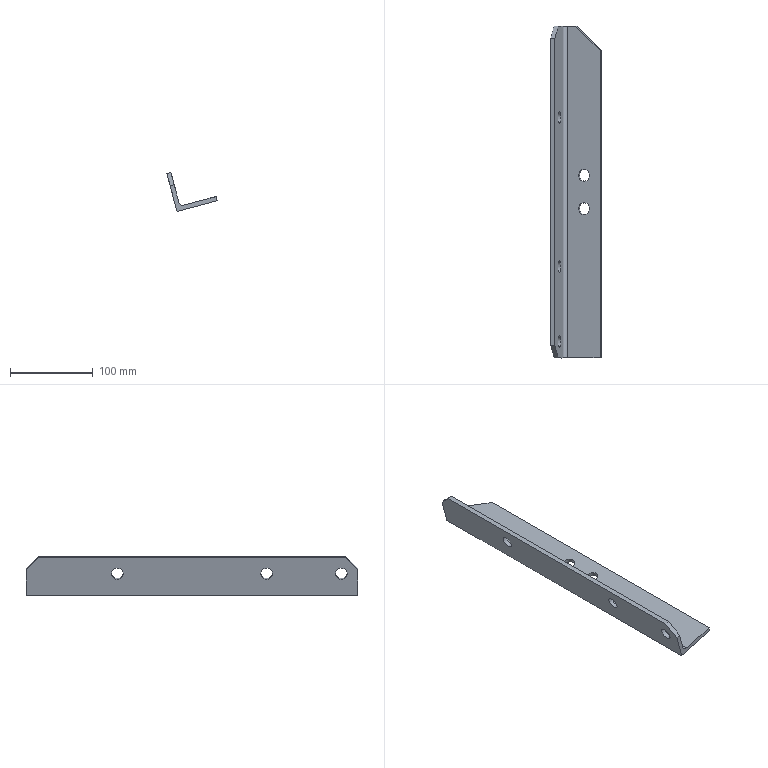Part | NX | features solid 2 | 1 solid | 17 faces | box 60.461 x 400 x 46.693 mm | volume 178923 mm3 | plane 11 | cylinder 6 | commonest cylinder face diameters 14 x5 10 x1
STEP:
#1=CARTESIAN_POINT('',(712.611,-855.,-13.897));
#2=VERTEX_POINT('',#1);
#3=CARTESIAN_POINT('',(719.373,-855.,-12.085));
#4=DIRECTION('',(0.2588,0.,-0.9659));
#5=DIRECTION('',(-0.9659,0.,-0.2588));
#6=AXIS2_PLACEMENT_3D('',#3,#4,#5);
#7=CIRCLE('',#6,7.);
#8=EDGE_CURVE('',#2,#2,#7,.T.);
#9=ORIENTED_EDGE('',*,*,#8,.T.);
#10=EDGE_LOOP('',(#9));
#11=FACE_BOUND('',#10,.T.);
#12=CARTESIAN_POINT('',(738.691,-665.,-6.909));
#13=VERTEX_POINT('',#12);
#14=CARTESIAN_POINT('',(738.691,-1035.,-6.909));
#15=VERTEX_POINT('',#14);
#16=CARTESIAN_POINT('',(738.691,-859.636,-6.909));
#17=DIRECTION('',(0.,-1.,0.));
#18=VECTOR('',#17,1000.);
#19=LINE('',#16,#18);
#20=EDGE_CURVE('',#13,#15,#19,.T.);
#21=ORIENTED_EDGE('',*,*,#20,.F.);
#22=CARTESIAN_POINT('',(709.713,-635.,-14.673));
#23=VERTEX_POINT('',#22);
#24=CARTESIAN_POINT('',(831.809,-761.403,18.042));
#25=DIRECTION('',(0.683,-0.7071,0.183));
#26=VECTOR('',#25,1000.);
#27=LINE('',#24,#26);
#28=EDGE_CURVE('',#13,#23,#27,.F.);
#29=ORIENTED_EDGE('',*,*,#28,.T.);
#30=CARTESIAN_POINT('',(700.054,-635.,-17.261));
#31=VERTEX_POINT('',#30);
#32=CARTESIAN_POINT('',(695.225,-635.,-18.555));
#33=DIRECTION('',(-0.9659,0.,-0.2588));
#34=VECTOR('',#33,1000.);
#35=LINE('',#32,#34);
#36=EDGE_CURVE('',#23,#31,#35,.T.);
#37=ORIENTED_EDGE('',*,*,#36,.T.);
#38=CARTESIAN_POINT('',(700.054,-1035.,-17.261));
#39=VERTEX_POINT('',#38);
#40=CARTESIAN_POINT('',(700.054,-740.,-17.261));
#41=DIRECTION('',(0.,-1.,0.));
#42=VECTOR('',#41,1000.);
#43=LINE('',#40,#42);
#44=EDGE_CURVE('',#39,#31,#43,.F.);
#45=ORIENTED_EDGE('',*,*,#44,.F.);
#46=CARTESIAN_POINT('',(738.691,-1035.,-6.909));
#47=DIRECTION('',(0.9659,0.,0.2588));
#48=VECTOR('',#47,1000.);
#49=LINE('',#46,#48);
#50=EDGE_CURVE('',#39,#15,#49,.T.);
#51=ORIENTED_EDGE('',*,*,#50,.T.);
#52=EDGE_LOOP('',(#21,#29,#37,#45,#51));
#53=FACE_BOUND('',#52,.T.);
#54=CARTESIAN_POINT('',(712.611,-815.,-13.897));
#55=VERTEX_POINT('',#54);
#56=CARTESIAN_POINT('',(719.373,-815.,-12.085));
#57=DIRECTION('',(0.2588,0.,-0.9659));
#58=DIRECTION('',(-0.9659,0.,-0.2588));
#59=AXIS2_PLACEMENT_3D('',#56,#57,#58);
#60=CIRCLE('',#59,7.);
#61=EDGE_CURVE('',#55,#55,#60,.T.);
#62=ORIENTED_EDGE('',*,*,#61,.T.);
#63=EDGE_LOOP('',(#62));
#64=FACE_BOUND('',#63,.T.);
#65=CARTESIAN_POINT('',(738.691,-857.805,-6.909));
#66=DIRECTION('',(-0.2588,0.,0.9659));
#67=DIRECTION('',(0.,-1.,0.));
#68=AXIS2_PLACEMENT_3D('',#65,#66,#67);
#69=PLANE('',#68);
#70=ADVANCED_FACE('',(#11,#53,#64),#69,.T.);
#71=CARTESIAN_POINT('',(713.905,-855.,-18.726));
#72=VERTEX_POINT('',#71);
#73=CARTESIAN_POINT('',(720.667,-855.,-16.915));
#74=DIRECTION('',(0.2588,0.,-0.9659));
#75=DIRECTION('',(-0.9659,0.,-0.2588));
#76=AXIS2_PLACEMENT_3D('',#73,#74,#75);
#77=CIRCLE('',#76,7.);
#78=EDGE_CURVE('',#72,#72,#77,.F.);
#79=ORIENTED_EDGE('',*,*,#78,.T.);
#80=EDGE_LOOP('',(#79));
#81=FACE_BOUND('',#80,.T.);
#82=CARTESIAN_POINT('',(691.689,-635.,-24.679));
#83=VERTEX_POINT('',#82);
#84=CARTESIAN_POINT('',(711.008,-635.,-19.503));
#85=VERTEX_POINT('',#84);
#86=CARTESIAN_POINT('',(696.519,-635.,-23.385));
#87=DIRECTION('',(0.9659,0.,0.2588));
#88=VECTOR('',#87,1000.);
#89=LINE('',#86,#88);
#90=EDGE_CURVE('',#83,#85,#89,.T.);
#91=ORIENTED_EDGE('',*,*,#90,.T.);
#92=CARTESIAN_POINT('',(739.985,-665.,-11.738));
#93=VERTEX_POINT('',#92);
#94=CARTESIAN_POINT('',(811.222,-738.75,7.35));
#95=DIRECTION('',(-0.683,0.7071,-0.183));
#96=VECTOR('',#95,1000.);
#97=LINE('',#94,#96);
#98=EDGE_CURVE('',#85,#93,#97,.F.);
#99=ORIENTED_EDGE('',*,*,#98,.T.);
#100=CARTESIAN_POINT('',(739.985,-1035.,-11.738));
#101=VERTEX_POINT('',#100);
#102=CARTESIAN_POINT('',(739.985,-857.5,-11.738));
#103=DIRECTION('',(0.,-1.,0.));
#104=VECTOR('',#103,1000.);
#105=LINE('',#102,#104);
#106=EDGE_CURVE('',#93,#101,#105,.T.);
#107=ORIENTED_EDGE('',*,*,#106,.T.);
#108=CARTESIAN_POINT('',(691.689,-1035.,-24.679));
#109=VERTEX_POINT('',#108);
#110=CARTESIAN_POINT('',(696.519,-1035.,-23.385));
#111=DIRECTION('',(-0.9659,0.,-0.2588));
#112=VECTOR('',#111,1000.);
#113=LINE('',#110,#112);
#114=EDGE_CURVE('',#101,#109,#113,.T.);
#115=ORIENTED_EDGE('',*,*,#114,.T.);
#116=CARTESIAN_POINT('',(691.689,-859.636,-24.679));
#117=DIRECTION('',(0.,-1.,0.));
#118=VECTOR('',#117,1000.);
#119=LINE('',#116,#118);
#120=EDGE_CURVE('',#83,#109,#119,.T.);
#121=ORIENTED_EDGE('',*,*,#120,.F.);
#122=EDGE_LOOP('',(#91,#99,#107,#115,#121));
#123=FACE_BOUND('',#122,.T.);
#124=CARTESIAN_POINT('',(713.905,-815.,-18.726));
#125=VERTEX_POINT('',#124);
#126=CARTESIAN_POINT('',(720.667,-815.,-16.915));
#127=DIRECTION('',(0.2588,0.,-0.9659));
#128=DIRECTION('',(-0.9659,0.,-0.2588));
#129=AXIS2_PLACEMENT_3D('',#126,#127,#128);
#130=CIRCLE('',#129,7.);
#131=EDGE_CURVE('',#125,#125,#130,.F.);
#132=ORIENTED_EDGE('',*,*,#131,.T.);
#133=EDGE_LOOP('',(#132));
#134=FACE_BOUND('',#133,.T.);
#135=CARTESIAN_POINT('',(696.519,-857.5,-23.385));
#136=DIRECTION('',(0.2588,0.,-0.9659));
#137=DIRECTION('',(0.,1.,0.));
#138=AXIS2_PLACEMENT_3D('',#135,#136,#137);
#139=PLANE('',#138);
#140=ADVANCED_FACE('',(#81,#123,#134),#139,.T.);
#141=CARTESIAN_POINT('',(691.342,-745.,-4.067));
#142=VERTEX_POINT('',#141);
#143=CARTESIAN_POINT('',(689.531,-745.,2.695));
#144=DIRECTION('',(0.9659,0.,0.2588));
#145=DIRECTION('',(0.2588,0.,-0.9659));
#146=AXIS2_PLACEMENT_3D('',#143,#144,#145);
#147=CIRCLE('',#146,7.);
#148=EDGE_CURVE('',#142,#142,#147,.F.);
#149=ORIENTED_EDGE('',*,*,#148,.T.);
#150=EDGE_LOOP('',(#149));
#151=FACE_BOUND('',#150,.T.);
#152=CARTESIAN_POINT('',(691.342,-925.,-4.067));
#153=VERTEX_POINT('',#152);
#154=CARTESIAN_POINT('',(689.531,-925.,2.695));
#155=DIRECTION('',(0.9659,0.,0.2588));
#156=DIRECTION('',(0.2588,0.,-0.9659));
#157=AXIS2_PLACEMENT_3D('',#154,#155,#156);
#158=CIRCLE('',#157,7.);
#159=EDGE_CURVE('',#153,#153,#158,.F.);
#160=ORIENTED_EDGE('',*,*,#159,.T.);
#161=EDGE_LOOP('',(#160));
#162=FACE_BOUND('',#161,.T.);
#163=CARTESIAN_POINT('',(688.236,-1035.,7.525));
#164=VERTEX_POINT('',#163);
#165=CARTESIAN_POINT('',(693.93,-1035.,-13.726));
#166=VERTEX_POINT('',#165);
#167=CARTESIAN_POINT('',(687.46,-1035.,10.422));
#168=DIRECTION('',(0.2588,0.,-0.9659));
#169=VECTOR('',#168,1000.);
#170=LINE('',#167,#169);
#171=EDGE_CURVE('',#164,#166,#170,.T.);
#172=ORIENTED_EDGE('',*,*,#171,.T.);
#173=CARTESIAN_POINT('',(693.93,-635.,-13.726));
#174=VERTEX_POINT('',#173);
#175=CARTESIAN_POINT('',(693.93,-1074.813,-13.726));
#176=DIRECTION('',(0.,-1.,0.));
#177=VECTOR('',#176,1000.);
#178=LINE('',#175,#177);
#179=EDGE_CURVE('',#174,#166,#178,.T.);
#180=ORIENTED_EDGE('',*,*,#179,.F.);
#181=CARTESIAN_POINT('',(688.236,-635.,7.525));
#182=VERTEX_POINT('',#181);
#183=CARTESIAN_POINT('',(689.531,-635.,2.695));
#184=DIRECTION('',(-0.2588,0.,0.9659));
#185=VECTOR('',#184,1000.);
#186=LINE('',#183,#185);
#187=EDGE_CURVE('',#174,#182,#186,.T.);
#188=ORIENTED_EDGE('',*,*,#187,.T.);
#189=CARTESIAN_POINT('',(684.354,-650.,22.013));
#190=VERTEX_POINT('',#189);
#191=CARTESIAN_POINT('',(670.425,-703.818,73.997));
#192=DIRECTION('',(-0.183,-0.7071,0.683));
#193=VECTOR('',#192,1000.);
#194=LINE('',#191,#193);
#195=EDGE_CURVE('',#190,#182,#194,.F.);
#196=ORIENTED_EDGE('',*,*,#195,.F.);
#197=CARTESIAN_POINT('',(684.354,-1020.,22.013));
#198=VERTEX_POINT('',#197);
#199=CARTESIAN_POINT('',(684.354,-859.636,22.013));
#200=DIRECTION('',(0.,-1.,0.));
#201=VECTOR('',#200,1000.);
#202=LINE('',#199,#201);
#203=EDGE_CURVE('',#190,#198,#202,.T.);
#204=ORIENTED_EDGE('',*,*,#203,.T.);
#205=CARTESIAN_POINT('',(665.154,-945.818,93.668));
#206=DIRECTION('',(-0.183,0.7071,0.683));
#207=VECTOR('',#206,1000.);
#208=LINE('',#205,#207);
#209=EDGE_CURVE('',#164,#198,#208,.T.);
#210=ORIENTED_EDGE('',*,*,#209,.F.);
#211=EDGE_LOOP('',(#172,#180,#188,#196,#204,#210));
#212=FACE_BOUND('',#211,.T.);
#213=CARTESIAN_POINT('',(687.719,-1015.,9.456));
#214=VERTEX_POINT('',#213);
#215=CARTESIAN_POINT('',(689.531,-1015.,2.695));
#216=DIRECTION('',(-0.9659,0.,-0.2588));
#217=DIRECTION('',(-0.2588,0.,0.9659));
#218=AXIS2_PLACEMENT_3D('',#215,#216,#217);
#219=CIRCLE('',#218,7.);
#220=EDGE_CURVE('',#214,#214,#219,.F.);
#221=ORIENTED_EDGE('',*,*,#220,.F.);
#222=EDGE_LOOP('',(#221));
#223=FACE_BOUND('',#222,.T.);
#224=CARTESIAN_POINT('',(687.46,-859.636,10.422));
#225=DIRECTION('',(0.9659,0.,0.2588));
#226=DIRECTION('',(0.2588,0.,-0.9659));
#227=AXIS2_PLACEMENT_3D('',#224,#225,#226);
#228=PLANE('',#227);
#229=ADVANCED_FACE('',(#151,#162,#212,#223),#228,.T.);
#230=CARTESIAN_POINT('',(682.889,-745.,8.162));
#231=VERTEX_POINT('',#230);
#232=CARTESIAN_POINT('',(684.701,-745.,1.401));
#233=DIRECTION('',(-0.9659,0.,-0.2588));
#234=DIRECTION('',(-0.2588,0.,0.9659));
#235=AXIS2_PLACEMENT_3D('',#232,#233,#234);
#236=CIRCLE('',#235,7.);
#237=EDGE_CURVE('',#231,#231,#236,.F.);
#238=ORIENTED_EDGE('',*,*,#237,.T.);
#239=EDGE_LOOP('',(#238));
#240=FACE_BOUND('',#239,.T.);
#241=CARTESIAN_POINT('',(682.889,-925.,8.162));
#242=VERTEX_POINT('',#241);
#243=CARTESIAN_POINT('',(684.701,-925.,1.401));
#244=DIRECTION('',(-0.9659,0.,-0.2588));
#245=DIRECTION('',(-0.2588,0.,0.9659));
#246=AXIS2_PLACEMENT_3D('',#243,#244,#245);
#247=CIRCLE('',#246,7.);
#248=EDGE_CURVE('',#242,#242,#247,.F.);
#249=ORIENTED_EDGE('',*,*,#248,.T.);
#250=EDGE_LOOP('',(#249));
#251=FACE_BOUND('',#250,.T.);
#252=CARTESIAN_POINT('',(679.525,-650.,20.719));
#253=VERTEX_POINT('',#252);
#254=CARTESIAN_POINT('',(679.525,-1020.,20.719));
#255=VERTEX_POINT('',#254);
#256=CARTESIAN_POINT('',(679.525,-859.636,20.719));
#257=DIRECTION('',(0.,-1.,0.));
#258=VECTOR('',#257,1000.);
#259=LINE('',#256,#258);
#260=EDGE_CURVE('',#253,#255,#259,.T.);
#261=ORIENTED_EDGE('',*,*,#260,.F.);
#262=CARTESIAN_POINT('',(683.407,-635.,6.23));
#263=VERTEX_POINT('',#262);
#264=CARTESIAN_POINT('',(665.595,-703.818,72.703));
#265=DIRECTION('',(0.183,0.7071,-0.683));
#266=VECTOR('',#265,1000.);
#267=LINE('',#264,#266);
#268=EDGE_CURVE('',#263,#253,#267,.F.);
#269=ORIENTED_EDGE('',*,*,#268,.F.);
#270=CARTESIAN_POINT('',(684.701,-635.,1.401));
#271=DIRECTION('',(0.2588,0.,-0.9659));
#272=VECTOR('',#271,1000.);
#273=LINE('',#270,#272);
#274=EDGE_CURVE('',#263,#83,#273,.T.);
#275=ORIENTED_EDGE('',*,*,#274,.T.);
#276=ORIENTED_EDGE('',*,*,#120,.T.);
#277=CARTESIAN_POINT('',(683.407,-1035.,6.23));
#278=VERTEX_POINT('',#277);
#279=CARTESIAN_POINT('',(682.63,-1035.,9.128));
#280=DIRECTION('',(-0.2588,0.,0.9659));
#281=VECTOR('',#280,1000.);
#282=LINE('',#279,#281);
#283=EDGE_CURVE('',#109,#278,#282,.T.);
#284=ORIENTED_EDGE('',*,*,#283,.T.);
#285=CARTESIAN_POINT('',(660.325,-945.818,92.374));
#286=DIRECTION('',(0.183,-0.7071,-0.683));
#287=VECTOR('',#286,1000.);
#288=LINE('',#285,#287);
#289=EDGE_CURVE('',#255,#278,#288,.T.);
#290=ORIENTED_EDGE('',*,*,#289,.F.);
#291=EDGE_LOOP('',(#261,#269,#275,#276,#284,#290));
#292=FACE_BOUND('',#291,.T.);
#293=CARTESIAN_POINT('',(686.513,-1015.,-5.361));
#294=VERTEX_POINT('',#293);
#295=CARTESIAN_POINT('',(684.701,-1015.,1.401));
#296=DIRECTION('',(0.9659,0.,0.2588));
#297=DIRECTION('',(0.2588,0.,-0.9659));
#298=AXIS2_PLACEMENT_3D('',#295,#296,#297);
#299=CIRCLE('',#298,7.);
#300=EDGE_CURVE('',#294,#294,#299,.T.);
#301=ORIENTED_EDGE('',*,*,#300,.T.);
#302=EDGE_LOOP('',(#301));
#303=FACE_BOUND('',#302,.T.);
#304=CARTESIAN_POINT('',(682.63,-859.636,9.128));
#305=DIRECTION('',(-0.9659,0.,-0.2588));
#306=DIRECTION('',(-0.2588,0.,0.9659));
#307=AXIS2_PLACEMENT_3D('',#304,#305,#306);
#308=PLANE('',#307);
#309=ADVANCED_FACE('',(#240,#251,#292,#303),#308,.T.);
#310=ORIENTED_EDGE('',*,*,#203,.F.);
#311=CARTESIAN_POINT('',(689.184,-650.,23.308));
#312=DIRECTION('',(0.9659,0.,0.2588));
#313=VECTOR('',#312,1000.);
#314=LINE('',#311,#313);
#315=EDGE_CURVE('',#253,#190,#314,.T.);
#316=ORIENTED_EDGE('',*,*,#315,.F.);
#317=ORIENTED_EDGE('',*,*,#260,.T.);
#318=CARTESIAN_POINT('',(679.525,-1020.,20.719));
#319=DIRECTION('',(-0.9659,0.,-0.2588));
#320=VECTOR('',#319,1000.);
#321=LINE('',#318,#320);
#322=EDGE_CURVE('',#198,#255,#321,.T.);
#323=ORIENTED_EDGE('',*,*,#322,.F.);
#324=EDGE_LOOP('',(#310,#316,#317,#323));
#325=FACE_BOUND('',#324,.T.);
#326=CARTESIAN_POINT('',(689.184,-859.636,23.308));
#327=DIRECTION('',(-0.2588,0.,0.9659));
#328=DIRECTION('',(0.,-1.,0.));
#329=AXIS2_PLACEMENT_3D('',#326,#327,#328);
#330=PLANE('',#329);
#331=ADVANCED_FACE('',(#325),#330,.T.);
#332=ORIENTED_EDGE('',*,*,#44,.T.);
#333=CARTESIAN_POINT('',(698.76,-635.,-12.432));
#334=DIRECTION('',(0.,-1.,0.));
#335=DIRECTION('',(0.9848,0.,-0.1736));
#336=AXIS2_PLACEMENT_3D('',#333,#334,#335);
#337=CIRCLE('',#336,5.);
#338=EDGE_CURVE('',#174,#31,#337,.T.);
#339=ORIENTED_EDGE('',*,*,#338,.F.);
#340=ORIENTED_EDGE('',*,*,#179,.T.);
#341=CARTESIAN_POINT('',(698.76,-1035.,-12.432));
#342=DIRECTION('',(0.,-1.,0.));
#343=DIRECTION('',(0.1736,0.,0.9848));
#344=AXIS2_PLACEMENT_3D('',#341,#342,#343);
#345=CIRCLE('',#344,5.);
#346=EDGE_CURVE('',#39,#166,#345,.F.);
#347=ORIENTED_EDGE('',*,*,#346,.F.);
#348=EDGE_LOOP('',(#332,#339,#340,#347));
#349=FACE_BOUND('',#348,.T.);
#350=CARTESIAN_POINT('',(698.76,-859.636,-12.432));
#351=DIRECTION('',(0.,1.,0.));
#352=DIRECTION('',(0.2588,0.,-0.9659));
#353=AXIS2_PLACEMENT_3D('',#350,#351,#352);
#354=CYLINDRICAL_SURFACE('',#353,5.);
#355=ADVANCED_FACE('',(#349),#354,.F.);
#356=ORIENTED_EDGE('',*,*,#106,.F.);
#357=CARTESIAN_POINT('',(730.927,-665.,22.069));
#358=DIRECTION('',(-0.2588,0.,0.9659));
#359=VECTOR('',#358,1000.);
#360=LINE('',#357,#359);
#361=EDGE_CURVE('',#93,#13,#360,.T.);
#362=ORIENTED_EDGE('',*,*,#361,.T.);
#363=ORIENTED_EDGE('',*,*,#20,.T.);
#364=CARTESIAN_POINT('',(730.927,-1035.,22.069));
#365=DIRECTION('',(0.2588,0.,-0.9659));
#366=VECTOR('',#365,1000.);
#367=LINE('',#364,#366);
#368=EDGE_CURVE('',#15,#101,#367,.T.);
#369=ORIENTED_EDGE('',*,*,#368,.T.);
#370=EDGE_LOOP('',(#356,#362,#363,#369));
#371=FACE_BOUND('',#370,.T.);
#372=CARTESIAN_POINT('',(730.927,-859.636,22.069));
#373=DIRECTION('',(0.9659,0.,0.2588));
#374=DIRECTION('',(0.2588,0.,-0.9659));
#375=AXIS2_PLACEMENT_3D('',#372,#373,#374);
#376=PLANE('',#375);
#377=ADVANCED_FACE('',(#371),#376,.T.);
#378=ORIENTED_EDGE('',*,*,#159,.F.);
#379=EDGE_LOOP('',(#378));
#380=FACE_BOUND('',#379,.T.);
#381=ORIENTED_EDGE('',*,*,#248,.F.);
#382=EDGE_LOOP('',(#381));
#383=FACE_BOUND('',#382,.T.);
#384=CARTESIAN_POINT('',(713.679,-925.,9.165));
#385=DIRECTION('',(-0.9659,0.,-0.2588));
#386=DIRECTION('',(0.,-1.,0.));
#387=AXIS2_PLACEMENT_3D('',#384,#385,#386);
#388=CYLINDRICAL_SURFACE('',#387,7.);
#389=ADVANCED_FACE('',(#380,#383),#388,.F.);
#390=ORIENTED_EDGE('',*,*,#283,.F.);
#391=ORIENTED_EDGE('',*,*,#114,.F.);
#392=ORIENTED_EDGE('',*,*,#368,.F.);
#393=ORIENTED_EDGE('',*,*,#50,.F.);
#394=ORIENTED_EDGE('',*,*,#346,.T.);
#395=ORIENTED_EDGE('',*,*,#171,.F.);
#396=CARTESIAN_POINT('',(688.236,-1035.,7.525));
#397=DIRECTION('',(0.9659,0.,0.2588));
#398=VECTOR('',#397,1000.);
#399=LINE('',#396,#398);
#400=EDGE_CURVE('',#278,#164,#399,.T.);
#401=ORIENTED_EDGE('',*,*,#400,.F.);
#402=EDGE_LOOP('',(#390,#391,#392,#393,#394,#395,#401));
#403=FACE_BOUND('',#402,.T.);
#404=CARTESIAN_POINT('',(103.71,-1035.,-64.317));
#405=DIRECTION('',(0.,1.,0.));
#406=DIRECTION('',(0.1736,0.,0.9848));
#407=AXIS2_PLACEMENT_3D('',#404,#405,#406);
#408=PLANE('',#407);
#409=ADVANCED_FACE('',(#403),#408,.F.);
#410=ORIENTED_EDGE('',*,*,#36,.F.);
#411=CARTESIAN_POINT('',(704.019,-635.,6.577));
#412=DIRECTION('',(0.2588,0.,-0.9659));
#413=VECTOR('',#412,1000.);
#414=LINE('',#411,#413);
#415=EDGE_CURVE('',#23,#85,#414,.T.);
#416=ORIENTED_EDGE('',*,*,#415,.T.);
#417=ORIENTED_EDGE('',*,*,#90,.F.);
#418=ORIENTED_EDGE('',*,*,#274,.F.);
#419=CARTESIAN_POINT('',(688.236,-635.,7.525));
#420=DIRECTION('',(-0.9659,0.,-0.2588));
#421=VECTOR('',#420,1000.);
#422=LINE('',#419,#421);
#423=EDGE_CURVE('',#182,#263,#422,.T.);
#424=ORIENTED_EDGE('',*,*,#423,.F.);
#425=ORIENTED_EDGE('',*,*,#187,.F.);
#426=ORIENTED_EDGE('',*,*,#338,.T.);
#427=EDGE_LOOP('',(#410,#416,#417,#418,#424,#425,#426));
#428=FACE_BOUND('',#427,.T.);
#429=CARTESIAN_POINT('',(689.531,-635.,2.695));
#430=DIRECTION('',(0.,1.,0.));
#431=DIRECTION('',(-0.766,0.,-0.6428));
#432=AXIS2_PLACEMENT_3D('',#429,#430,#431);
#433=PLANE('',#432);
#434=ADVANCED_FACE('',(#428),#433,.T.);
#435=ORIENTED_EDGE('',*,*,#148,.F.);
#436=EDGE_LOOP('',(#435));
#437=FACE_BOUND('',#436,.T.);
#438=ORIENTED_EDGE('',*,*,#237,.F.);
#439=EDGE_LOOP('',(#438));
#440=FACE_BOUND('',#439,.T.);
#441=CARTESIAN_POINT('',(713.679,-745.,9.165));
#442=DIRECTION('',(-0.9659,0.,-0.2588));
#443=DIRECTION('',(0.,-1.,0.));
#444=AXIS2_PLACEMENT_3D('',#441,#442,#443);
#445=CYLINDRICAL_SURFACE('',#444,7.);
#446=ADVANCED_FACE('',(#437,#440),#445,.F.);
#447=ORIENTED_EDGE('',*,*,#220,.T.);
#448=EDGE_LOOP('',(#447));
#449=FACE_BOUND('',#448,.T.);
#450=ORIENTED_EDGE('',*,*,#300,.F.);
#451=EDGE_LOOP('',(#450));
#452=FACE_BOUND('',#451,.T.);
#453=CARTESIAN_POINT('',(713.679,-1015.,9.165));
#454=DIRECTION('',(-0.9659,0.,-0.2588));
#455=DIRECTION('',(0.,-1.,0.));
#456=AXIS2_PLACEMENT_3D('',#453,#454,#455);
#457=CYLINDRICAL_SURFACE('',#456,7.);
#458=ADVANCED_FACE('',(#449,#452),#457,.F.);
#459=ORIENTED_EDGE('',*,*,#289,.T.);
#460=ORIENTED_EDGE('',*,*,#400,.T.);
#461=ORIENTED_EDGE('',*,*,#209,.T.);
#462=ORIENTED_EDGE('',*,*,#322,.T.);
#463=EDGE_LOOP('',(#459,#460,#461,#462));
#464=FACE_BOUND('',#463,.T.);
#465=CARTESIAN_POINT('',(124.906,-1035.,-143.419));
#466=DIRECTION('',(-0.183,-0.7071,0.683));
#467=DIRECTION('',(-0.1287,-0.6715,-0.7297));
#468=AXIS2_PLACEMENT_3D('',#465,#466,#467);
#469=PLANE('',#468);
#470=ADVANCED_FACE('',(#464),#469,.T.);
#471=ORIENTED_EDGE('',*,*,#195,.T.);
#472=ORIENTED_EDGE('',*,*,#423,.T.);
#473=ORIENTED_EDGE('',*,*,#268,.T.);
#474=ORIENTED_EDGE('',*,*,#315,.T.);
#475=EDGE_LOOP('',(#471,#472,#473,#474));
#476=FACE_BOUND('',#475,.T.);
#477=CARTESIAN_POINT('',(688.236,-635.,7.525));
#478=DIRECTION('',(0.183,-0.7071,-0.683));
#479=DIRECTION('',(-0.1287,0.6715,-0.7297));
#480=AXIS2_PLACEMENT_3D('',#477,#478,#479);
#481=PLANE('',#480);
#482=ADVANCED_FACE('',(#476),#481,.F.);
#483=ORIENTED_EDGE('',*,*,#78,.F.);
#484=EDGE_LOOP('',(#483));
#485=FACE_BOUND('',#484,.T.);
#486=ORIENTED_EDGE('',*,*,#8,.F.);
#487=EDGE_LOOP('',(#486));
#488=FACE_BOUND('',#487,.T.);
#489=CARTESIAN_POINT('',(732.314,-855.,-60.381));
#490=DIRECTION('',(-0.2588,0.,0.9659));
#491=DIRECTION('',(-0.9659,0.,-0.2588));
#492=AXIS2_PLACEMENT_3D('',#489,#490,#491);
#493=CYLINDRICAL_SURFACE('',#492,7.);
#494=ADVANCED_FACE('',(#485,#488),#493,.F.);
#495=ORIENTED_EDGE('',*,*,#131,.F.);
#496=EDGE_LOOP('',(#495));
#497=FACE_BOUND('',#496,.T.);
#498=ORIENTED_EDGE('',*,*,#61,.F.);
#499=EDGE_LOOP('',(#498));
#500=FACE_BOUND('',#499,.T.);
#501=CARTESIAN_POINT('',(732.314,-815.,-60.381));
#502=DIRECTION('',(-0.2588,0.,0.9659));
#503=DIRECTION('',(-0.9659,0.,-0.2588));
#504=AXIS2_PLACEMENT_3D('',#501,#502,#503);
#505=CYLINDRICAL_SURFACE('',#504,7.);
#506=ADVANCED_FACE('',(#497,#500),#505,.F.);
#507=ORIENTED_EDGE('',*,*,#98,.F.);
#508=ORIENTED_EDGE('',*,*,#415,.F.);
#509=ORIENTED_EDGE('',*,*,#28,.F.);
#510=ORIENTED_EDGE('',*,*,#361,.F.);
#511=EDGE_LOOP('',(#507,#508,#509,#510));
#512=FACE_BOUND('',#511,.T.);
#513=CARTESIAN_POINT('',(730.927,-665.,22.069));
#514=DIRECTION('',(-0.683,-0.7071,-0.183));
#515=DIRECTION('',(0.7193,-0.6947,0.));
#516=AXIS2_PLACEMENT_3D('',#513,#514,#515);
#517=PLANE('',#516);
#518=ADVANCED_FACE('',(#512),#517,.F.);
#519=CLOSED_SHELL('',(#70,#140,#229,#309,#331,#355,#377,#389,#409,#434,#446,#458,#470,#482,#494,#506,#518));
#520=MANIFOLD_SOLID_BREP('',#519);
#521=(LENGTH_UNIT()NAMED_UNIT(*)SI_UNIT(.MILLI.,.METRE.));
#522=UNCERTAINTY_MEASURE_WITH_UNIT(LENGTH_MEASURE(0.00001),#521,'','');
#523=(NAMED_UNIT(*)PLANE_ANGLE_UNIT()SI_UNIT($,.RADIAN.));
#524=(NAMED_UNIT(*)SI_UNIT($,.STERADIAN.)SOLID_ANGLE_UNIT());
#525=(GEOMETRIC_REPRESENTATION_CONTEXT(3)GLOBAL_UNCERTAINTY_ASSIGNED_CONTEXT((#522))GLOBAL_UNIT_ASSIGNED_CONTEXT((#521,#523,#524))REPRESENTATION_CONTEXT('',''));
#526=ADVANCED_BREP_SHAPE_REPRESENTATION('',(#520),#525);